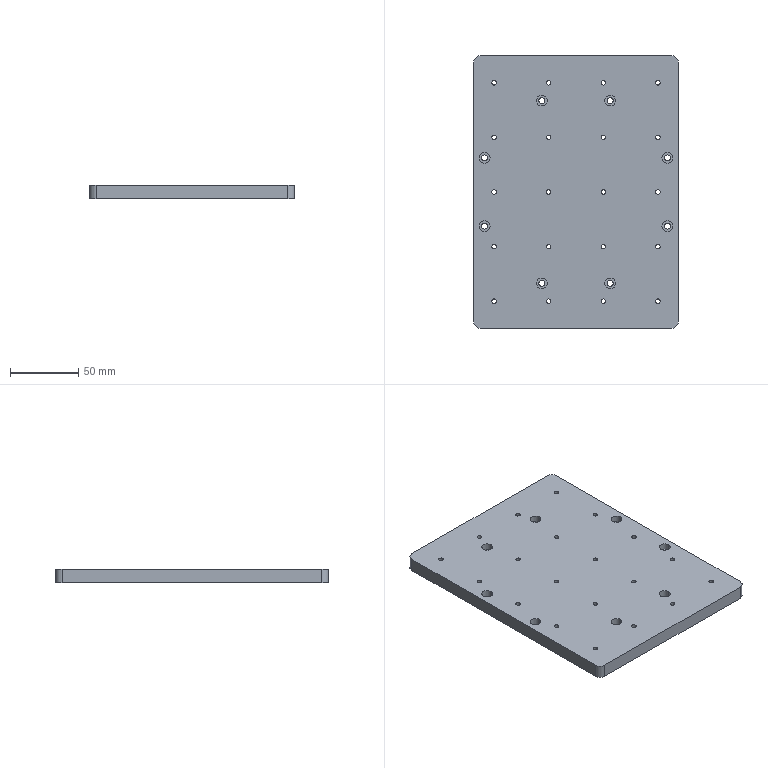Part | SolidWorks | features HoleWzd 3, ICE 3, Extrusion 1, Fillet 1, LPattern 1 | 1 solid | 90 faces | box 150 x 200 x 10 mm | volume 295428 mm3 | cylinder 76 | plane 14 | commonest cylinder face diameters 3.3 x40 4.5 x16 8 x16 10 x4